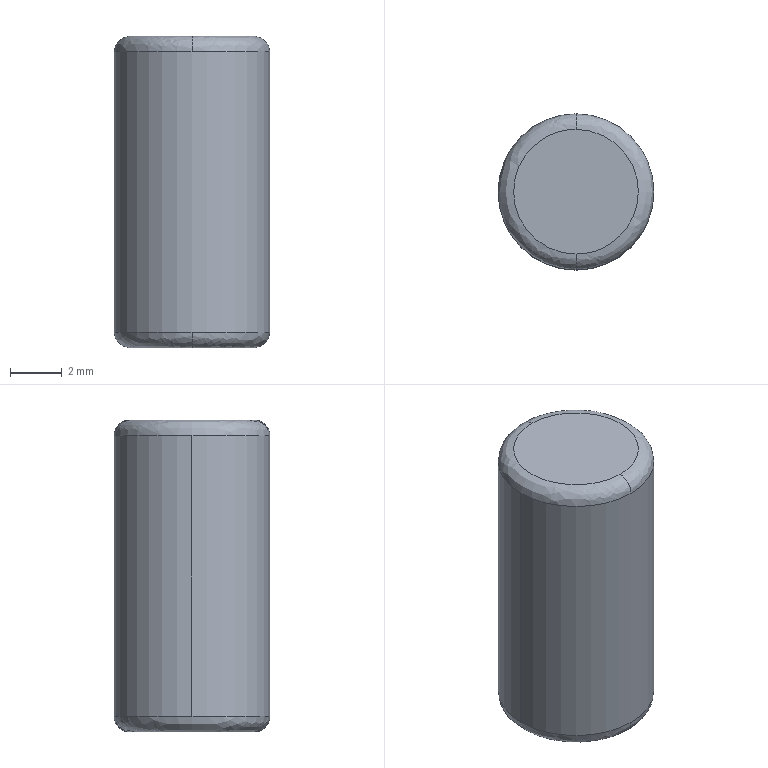Part | SolidWorks | features BaseBody 1 | 1 solid | 8 faces | box 6 x 6 x 12 mm | volume 336.497 mm3 | spline 4 | cylinder 2 | plane 2 | commonest cylinder face diameters 6 x2
STEP:
#1=CARTESIAN_POINT('',(442.747,1086.806,-452.745));
#2=VERTEX_POINT('',#1);
#3=CARTESIAN_POINT('',(445.747,1089.806,-452.745));
#4=VERTEX_POINT('',#3);
#5=CARTESIAN_POINT('',(442.747,1089.806,-452.745));
#6=DIRECTION('',(0.,0.,1.));
#7=DIRECTION('',(-1.,0.,0.));
#8=AXIS2_PLACEMENT_3D('',#5,#6,#7);
#9=CIRCLE('',#8,3.);
#10=EDGE_CURVE('',#2,#4,#9,.T.);
#11=ORIENTED_EDGE('',*,*,#10,.F.);
#12=CARTESIAN_POINT('',(442.747,1087.406,-453.345));
#13=VERTEX_POINT('',#12);
#14=CARTESIAN_POINT('',(442.747,1087.406,-452.745));
#15=DIRECTION('',(1.,0.,0.));
#16=DIRECTION('',(0.,-1.,0.));
#17=AXIS2_PLACEMENT_3D('',#14,#15,#16);
#18=CIRCLE('',#17,0.6);
#19=EDGE_CURVE('',#2,#13,#18,.T.);
#20=ORIENTED_EDGE('',*,*,#19,.T.);
#21=CARTESIAN_POINT('',(442.747,1092.206,-453.345));
#22=VERTEX_POINT('',#21);
#23=CARTESIAN_POINT('',(442.747,1087.406,-453.345));
#24=CARTESIAN_POINT('',(447.547,1087.406,-453.345));
#25=CARTESIAN_POINT('',(447.547,1092.206,-453.345));
#26=CARTESIAN_POINT('',(442.747,1092.206,-453.345));
#27=(BOUNDED_CURVE()B_SPLINE_CURVE(3,(#23,#24,#25,#26),.UNSPECIFIED.,.F.,.F.)B_SPLINE_CURVE_WITH_KNOTS((4,4),(0.,1.),.UNSPECIFIED.)CURVE()GEOMETRIC_REPRESENTATION_ITEM()RATIONAL_B_SPLINE_CURVE((1.,0.3333,0.3333,1.))REPRESENTATION_ITEM(''));
#28=EDGE_CURVE('',#13,#22,#27,.T.);
#29=ORIENTED_EDGE('',*,*,#28,.T.);
#30=CARTESIAN_POINT('',(442.747,1092.806,-452.745));
#31=VERTEX_POINT('',#30);
#32=CARTESIAN_POINT('',(442.747,1092.206,-452.745));
#33=DIRECTION('',(-1.,0.,0.));
#34=DIRECTION('',(0.,1.,0.));
#35=AXIS2_PLACEMENT_3D('',#32,#33,#34);
#36=CIRCLE('',#35,0.6);
#37=EDGE_CURVE('',#31,#22,#36,.T.);
#38=ORIENTED_EDGE('',*,*,#37,.F.);
#39=CARTESIAN_POINT('',(442.747,1089.806,-452.745));
#40=DIRECTION('',(0.,0.,1.));
#41=DIRECTION('',(-1.,0.,0.));
#42=AXIS2_PLACEMENT_3D('',#39,#40,#41);
#43=CIRCLE('',#42,3.);
#44=EDGE_CURVE('',#4,#31,#43,.T.);
#45=ORIENTED_EDGE('',*,*,#44,.F.);
#46=EDGE_LOOP('',(#11,#20,#29,#38,#45));
#47=FACE_OUTER_BOUND('',#46,.T.);
#48=CARTESIAN_POINT('',(442.747,1086.806,-452.745));
#49=CARTESIAN_POINT('',(448.747,1086.806,-452.745));
#50=CARTESIAN_POINT('',(448.747,1092.806,-452.745));
#51=CARTESIAN_POINT('',(442.747,1092.806,-452.745));
#52=CARTESIAN_POINT('',(442.747,1086.806,-453.096));
#53=CARTESIAN_POINT('',(448.747,1086.806,-453.096));
#54=CARTESIAN_POINT('',(448.747,1092.806,-453.096));
#55=CARTESIAN_POINT('',(442.747,1092.806,-453.096));
#56=CARTESIAN_POINT('',(442.747,1087.054,-453.345));
#57=CARTESIAN_POINT('',(448.249,1087.054,-453.345));
#58=CARTESIAN_POINT('',(448.249,1092.557,-453.345));
#59=CARTESIAN_POINT('',(442.747,1092.557,-453.345));
#60=CARTESIAN_POINT('',(442.747,1087.406,-453.345));
#61=CARTESIAN_POINT('',(447.547,1087.406,-453.345));
#62=CARTESIAN_POINT('',(447.547,1092.206,-453.345));
#63=CARTESIAN_POINT('',(442.747,1092.206,-453.345));
#64=(BOUNDED_SURFACE()B_SPLINE_SURFACE(3,3,((#48,#49,#50,#51),(#52,#53,#54,#55),(#56,#57,#58,#59),(#60,#61,#62,#63)),.UNSPECIFIED.,.F.,.F.,.F.)B_SPLINE_SURFACE_WITH_KNOTS((4,4),(4,4),(0.,1.),(0.,1.),.UNSPECIFIED.)GEOMETRIC_REPRESENTATION_ITEM()RATIONAL_B_SPLINE_SURFACE(((1.,0.3333,0.3333,1.),(0.8047,0.2682,0.2682,0.8047),(0.8047,0.2682,0.2682,0.8047),(1.,0.3333,0.3333,1.)))REPRESENTATION_ITEM('')SURFACE());
#65=ADVANCED_FACE('',(#47),#64,.T.);
#66=CARTESIAN_POINT('',(442.747,1092.206,-441.345));
#67=VERTEX_POINT('',#66);
#68=CARTESIAN_POINT('',(442.747,1087.406,-441.345));
#69=VERTEX_POINT('',#68);
#70=CARTESIAN_POINT('',(442.747,1092.206,-441.345));
#71=CARTESIAN_POINT('',(447.547,1092.206,-441.345));
#72=CARTESIAN_POINT('',(447.547,1087.406,-441.345));
#73=CARTESIAN_POINT('',(442.747,1087.406,-441.345));
#74=(BOUNDED_CURVE()B_SPLINE_CURVE(3,(#70,#71,#72,#73),.UNSPECIFIED.,.F.,.F.)B_SPLINE_CURVE_WITH_KNOTS((4,4),(0.,1.),.UNSPECIFIED.)CURVE()GEOMETRIC_REPRESENTATION_ITEM()RATIONAL_B_SPLINE_CURVE((1.,0.3333,0.3333,1.))REPRESENTATION_ITEM(''));
#75=EDGE_CURVE('',#67,#69,#74,.T.);
#76=ORIENTED_EDGE('',*,*,#75,.T.);
#77=CARTESIAN_POINT('',(442.747,1086.806,-441.945));
#78=VERTEX_POINT('',#77);
#79=CARTESIAN_POINT('',(442.747,1087.406,-441.945));
#80=DIRECTION('',(1.,0.,0.));
#81=DIRECTION('',(0.,-1.,0.));
#82=AXIS2_PLACEMENT_3D('',#79,#80,#81);
#83=CIRCLE('',#82,0.6);
#84=EDGE_CURVE('',#69,#78,#83,.T.);
#85=ORIENTED_EDGE('',*,*,#84,.T.);
#86=CARTESIAN_POINT('',(445.747,1089.806,-441.945));
#87=VERTEX_POINT('',#86);
#88=CARTESIAN_POINT('',(442.747,1089.806,-441.945));
#89=DIRECTION('',(0.,0.,-1.));
#90=DIRECTION('',(-1.,0.,0.));
#91=AXIS2_PLACEMENT_3D('',#88,#89,#90);
#92=CIRCLE('',#91,3.);
#93=EDGE_CURVE('',#87,#78,#92,.T.);
#94=ORIENTED_EDGE('',*,*,#93,.F.);
#95=CARTESIAN_POINT('',(442.747,1092.806,-441.945));
#96=VERTEX_POINT('',#95);
#97=CARTESIAN_POINT('',(442.747,1089.806,-441.945));
#98=DIRECTION('',(0.,0.,-1.));
#99=DIRECTION('',(-1.,0.,0.));
#100=AXIS2_PLACEMENT_3D('',#97,#98,#99);
#101=CIRCLE('',#100,3.);
#102=EDGE_CURVE('',#96,#87,#101,.T.);
#103=ORIENTED_EDGE('',*,*,#102,.F.);
#104=CARTESIAN_POINT('',(442.747,1092.206,-441.945));
#105=DIRECTION('',(-1.,0.,0.));
#106=DIRECTION('',(0.,1.,0.));
#107=AXIS2_PLACEMENT_3D('',#104,#105,#106);
#108=CIRCLE('',#107,0.6);
#109=EDGE_CURVE('',#67,#96,#108,.T.);
#110=ORIENTED_EDGE('',*,*,#109,.F.);
#111=EDGE_LOOP('',(#76,#85,#94,#103,#110));
#112=FACE_OUTER_BOUND('',#111,.T.);
#113=CARTESIAN_POINT('',(442.747,1087.406,-441.345));
#114=CARTESIAN_POINT('',(447.547,1087.406,-441.345));
#115=CARTESIAN_POINT('',(447.547,1092.206,-441.345));
#116=CARTESIAN_POINT('',(442.747,1092.206,-441.345));
#117=CARTESIAN_POINT('',(442.747,1087.054,-441.345));
#118=CARTESIAN_POINT('',(448.249,1087.054,-441.345));
#119=CARTESIAN_POINT('',(448.249,1092.557,-441.345));
#120=CARTESIAN_POINT('',(442.747,1092.557,-441.345));
#121=CARTESIAN_POINT('',(442.747,1086.806,-441.593));
#122=CARTESIAN_POINT('',(448.747,1086.806,-441.593));
#123=CARTESIAN_POINT('',(448.747,1092.806,-441.593));
#124=CARTESIAN_POINT('',(442.747,1092.806,-441.593));
#125=CARTESIAN_POINT('',(442.747,1086.806,-441.945));
#126=CARTESIAN_POINT('',(448.747,1086.806,-441.945));
#127=CARTESIAN_POINT('',(448.747,1092.806,-441.945));
#128=CARTESIAN_POINT('',(442.747,1092.806,-441.945));
#129=(BOUNDED_SURFACE()B_SPLINE_SURFACE(3,3,((#113,#114,#115,#116),(#117,#118,#119,#120),(#121,#122,#123,#124),(#125,#126,#127,#128)),.UNSPECIFIED.,.F.,.F.,.F.)B_SPLINE_SURFACE_WITH_KNOTS((4,4),(4,4),(0.,1.),(0.,1.),.UNSPECIFIED.)GEOMETRIC_REPRESENTATION_ITEM()RATIONAL_B_SPLINE_SURFACE(((1.,0.3333,0.3333,1.),(0.8047,0.2682,0.2682,0.8047),(0.8047,0.2682,0.2682,0.8047),(1.,0.3333,0.3333,1.)))REPRESENTATION_ITEM('')SURFACE());
#130=ADVANCED_FACE('',(#112),#129,.T.);
#131=CARTESIAN_POINT('',(439.747,1089.806,-441.945));
#132=VERTEX_POINT('',#131);
#133=CARTESIAN_POINT('',(442.747,1089.806,-441.945));
#134=DIRECTION('',(0.,0.,-1.));
#135=DIRECTION('',(-1.,0.,0.));
#136=AXIS2_PLACEMENT_3D('',#133,#134,#135);
#137=CIRCLE('',#136,3.);
#138=EDGE_CURVE('',#132,#96,#137,.T.);
#139=ORIENTED_EDGE('',*,*,#138,.T.);
#140=ORIENTED_EDGE('',*,*,#102,.T.);
#141=CARTESIAN_POINT('',(445.747,1089.806,-441.345));
#142=DIRECTION('',(0.,0.,-1.));
#143=VECTOR('',#142,1000.);
#144=LINE('',#141,#143);
#145=EDGE_CURVE('',#87,#4,#144,.T.);
#146=ORIENTED_EDGE('',*,*,#145,.T.);
#147=ORIENTED_EDGE('',*,*,#44,.T.);
#148=CARTESIAN_POINT('',(439.747,1089.806,-452.745));
#149=VERTEX_POINT('',#148);
#150=CARTESIAN_POINT('',(442.747,1089.806,-452.745));
#151=DIRECTION('',(0.,0.,1.));
#152=DIRECTION('',(-1.,0.,0.));
#153=AXIS2_PLACEMENT_3D('',#150,#151,#152);
#154=CIRCLE('',#153,3.);
#155=EDGE_CURVE('',#31,#149,#154,.T.);
#156=ORIENTED_EDGE('',*,*,#155,.T.);
#157=CARTESIAN_POINT('',(439.747,1089.806,-441.345));
#158=DIRECTION('',(0.,0.,-1.));
#159=VECTOR('',#158,1000.);
#160=LINE('',#157,#159);
#161=EDGE_CURVE('',#132,#149,#160,.T.);
#162=ORIENTED_EDGE('',*,*,#161,.F.);
#163=EDGE_LOOP('',(#139,#140,#146,#147,#156,#162));
#164=FACE_OUTER_BOUND('',#163,.T.);
#165=CARTESIAN_POINT('',(442.747,1089.806,-441.345));
#166=DIRECTION('',(0.,0.,-1.));
#167=DIRECTION('',(-1.,0.,0.));
#168=AXIS2_PLACEMENT_3D('',#165,#166,#167);
#169=CYLINDRICAL_SURFACE('',#168,3.);
#170=ADVANCED_FACE('',(#164),#169,.T.);
#171=ORIENTED_EDGE('',*,*,#145,.F.);
#172=ORIENTED_EDGE('',*,*,#93,.T.);
#173=CARTESIAN_POINT('',(442.747,1089.806,-441.945));
#174=DIRECTION('',(0.,0.,-1.));
#175=DIRECTION('',(-1.,0.,0.));
#176=AXIS2_PLACEMENT_3D('',#173,#174,#175);
#177=CIRCLE('',#176,3.);
#178=EDGE_CURVE('',#78,#132,#177,.T.);
#179=ORIENTED_EDGE('',*,*,#178,.T.);
#180=ORIENTED_EDGE('',*,*,#161,.T.);
#181=CARTESIAN_POINT('',(442.747,1089.806,-452.745));
#182=DIRECTION('',(0.,0.,1.));
#183=DIRECTION('',(-1.,0.,0.));
#184=AXIS2_PLACEMENT_3D('',#181,#182,#183);
#185=CIRCLE('',#184,3.);
#186=EDGE_CURVE('',#149,#2,#185,.T.);
#187=ORIENTED_EDGE('',*,*,#186,.T.);
#188=ORIENTED_EDGE('',*,*,#10,.T.);
#189=EDGE_LOOP('',(#171,#172,#179,#180,#187,#188));
#190=FACE_OUTER_BOUND('',#189,.T.);
#191=CARTESIAN_POINT('',(442.747,1089.806,-441.345));
#192=DIRECTION('',(0.,0.,-1.));
#193=DIRECTION('',(-1.,0.,0.));
#194=AXIS2_PLACEMENT_3D('',#191,#192,#193);
#195=CYLINDRICAL_SURFACE('',#194,3.);
#196=ADVANCED_FACE('',(#190),#195,.T.);
#197=ORIENTED_EDGE('',*,*,#19,.F.);
#198=ORIENTED_EDGE('',*,*,#186,.F.);
#199=ORIENTED_EDGE('',*,*,#155,.F.);
#200=ORIENTED_EDGE('',*,*,#37,.T.);
#201=CARTESIAN_POINT('',(442.747,1092.206,-453.345));
#202=CARTESIAN_POINT('',(437.947,1092.206,-453.345));
#203=CARTESIAN_POINT('',(437.947,1087.406,-453.345));
#204=CARTESIAN_POINT('',(442.747,1087.406,-453.345));
#205=(BOUNDED_CURVE()B_SPLINE_CURVE(3,(#201,#202,#203,#204),.UNSPECIFIED.,.F.,.F.)B_SPLINE_CURVE_WITH_KNOTS((4,4),(0.,1.),.UNSPECIFIED.)CURVE()GEOMETRIC_REPRESENTATION_ITEM()RATIONAL_B_SPLINE_CURVE((1.,0.3333,0.3333,1.))REPRESENTATION_ITEM(''));
#206=EDGE_CURVE('',#22,#13,#205,.T.);
#207=ORIENTED_EDGE('',*,*,#206,.T.);
#208=EDGE_LOOP('',(#197,#198,#199,#200,#207));
#209=FACE_OUTER_BOUND('',#208,.T.);
#210=CARTESIAN_POINT('',(442.747,1092.806,-452.745));
#211=CARTESIAN_POINT('',(436.747,1092.806,-452.745));
#212=CARTESIAN_POINT('',(436.747,1086.806,-452.745));
#213=CARTESIAN_POINT('',(442.747,1086.806,-452.745));
#214=CARTESIAN_POINT('',(442.747,1092.806,-453.096));
#215=CARTESIAN_POINT('',(436.747,1092.806,-453.096));
#216=CARTESIAN_POINT('',(436.747,1086.806,-453.096));
#217=CARTESIAN_POINT('',(442.747,1086.806,-453.096));
#218=CARTESIAN_POINT('',(442.747,1092.557,-453.345));
#219=CARTESIAN_POINT('',(437.244,1092.557,-453.345));
#220=CARTESIAN_POINT('',(437.244,1087.054,-453.345));
#221=CARTESIAN_POINT('',(442.747,1087.054,-453.345));
#222=CARTESIAN_POINT('',(442.747,1092.206,-453.345));
#223=CARTESIAN_POINT('',(437.947,1092.206,-453.345));
#224=CARTESIAN_POINT('',(437.947,1087.406,-453.345));
#225=CARTESIAN_POINT('',(442.747,1087.406,-453.345));
#226=(BOUNDED_SURFACE()B_SPLINE_SURFACE(3,3,((#210,#211,#212,#213),(#214,#215,#216,#217),(#218,#219,#220,#221),(#222,#223,#224,#225)),.UNSPECIFIED.,.F.,.F.,.T.)B_SPLINE_SURFACE_WITH_KNOTS((4,4),(4,4),(0.,1.),(0.,1.),.UNSPECIFIED.)GEOMETRIC_REPRESENTATION_ITEM()RATIONAL_B_SPLINE_SURFACE(((1.,0.3333,0.3333,1.),(0.8047,0.2682,0.2682,0.8047),(0.8047,0.2682,0.2682,0.8047),(1.,0.3333,0.3333,1.)))REPRESENTATION_ITEM('')SURFACE());
#227=ADVANCED_FACE('',(#209),#226,.T.);
#228=ORIENTED_EDGE('',*,*,#84,.F.);
#229=CARTESIAN_POINT('',(442.747,1087.406,-441.345));
#230=CARTESIAN_POINT('',(437.947,1087.406,-441.345));
#231=CARTESIAN_POINT('',(437.947,1092.206,-441.345));
#232=CARTESIAN_POINT('',(442.747,1092.206,-441.345));
#233=(BOUNDED_CURVE()B_SPLINE_CURVE(3,(#229,#230,#231,#232),.UNSPECIFIED.,.F.,.T.)B_SPLINE_CURVE_WITH_KNOTS((4,4),(0.,1.),.UNSPECIFIED.)CURVE()GEOMETRIC_REPRESENTATION_ITEM()RATIONAL_B_SPLINE_CURVE((1.,0.3333,0.3333,1.))REPRESENTATION_ITEM(''));
#234=EDGE_CURVE('',#69,#67,#233,.T.);
#235=ORIENTED_EDGE('',*,*,#234,.T.);
#236=ORIENTED_EDGE('',*,*,#109,.T.);
#237=ORIENTED_EDGE('',*,*,#138,.F.);
#238=ORIENTED_EDGE('',*,*,#178,.F.);
#239=EDGE_LOOP('',(#228,#235,#236,#237,#238));
#240=FACE_OUTER_BOUND('',#239,.T.);
#241=CARTESIAN_POINT('',(442.747,1092.206,-441.345));
#242=CARTESIAN_POINT('',(437.947,1092.206,-441.345));
#243=CARTESIAN_POINT('',(437.947,1087.406,-441.345));
#244=CARTESIAN_POINT('',(442.747,1087.406,-441.345));
#245=CARTESIAN_POINT('',(442.747,1092.557,-441.345));
#246=CARTESIAN_POINT('',(437.244,1092.557,-441.345));
#247=CARTESIAN_POINT('',(437.244,1087.054,-441.345));
#248=CARTESIAN_POINT('',(442.747,1087.054,-441.345));
#249=CARTESIAN_POINT('',(442.747,1092.806,-441.593));
#250=CARTESIAN_POINT('',(436.747,1092.806,-441.593));
#251=CARTESIAN_POINT('',(436.747,1086.806,-441.593));
#252=CARTESIAN_POINT('',(442.747,1086.806,-441.593));
#253=CARTESIAN_POINT('',(442.747,1092.806,-441.945));
#254=CARTESIAN_POINT('',(436.747,1092.806,-441.945));
#255=CARTESIAN_POINT('',(436.747,1086.806,-441.945));
#256=CARTESIAN_POINT('',(442.747,1086.806,-441.945));
#257=(BOUNDED_SURFACE()B_SPLINE_SURFACE(3,3,((#241,#242,#243,#244),(#245,#246,#247,#248),(#249,#250,#251,#252),(#253,#254,#255,#256)),.UNSPECIFIED.,.F.,.F.,.T.)B_SPLINE_SURFACE_WITH_KNOTS((4,4),(4,4),(0.,1.),(0.,1.),.UNSPECIFIED.)GEOMETRIC_REPRESENTATION_ITEM()RATIONAL_B_SPLINE_SURFACE(((1.,0.3333,0.3333,1.),(0.8047,0.2682,0.2682,0.8047),(0.8047,0.2682,0.2682,0.8047),(1.,0.3333,0.3333,1.)))REPRESENTATION_ITEM('')SURFACE());
#258=ADVANCED_FACE('',(#240),#257,.T.);
#259=ORIENTED_EDGE('',*,*,#28,.F.);
#260=ORIENTED_EDGE('',*,*,#206,.F.);
#261=EDGE_LOOP('',(#259,#260));
#262=FACE_OUTER_BOUND('',#261,.T.);
#263=CARTESIAN_POINT('',(442.747,1089.806,-453.345));
#264=DIRECTION('',(0.,0.,1.));
#265=DIRECTION('',(1.,0.,0.));
#266=AXIS2_PLACEMENT_3D('',#263,#264,#265);
#267=PLANE('',#266);
#268=ADVANCED_FACE('',(#262),#267,.F.);
#269=ORIENTED_EDGE('',*,*,#75,.F.);
#270=ORIENTED_EDGE('',*,*,#234,.F.);
#271=EDGE_LOOP('',(#269,#270));
#272=FACE_OUTER_BOUND('',#271,.T.);
#273=CARTESIAN_POINT('',(442.747,1089.806,-441.345));
#274=DIRECTION('',(0.,0.,1.));
#275=DIRECTION('',(1.,0.,0.));
#276=AXIS2_PLACEMENT_3D('',#273,#274,#275);
#277=PLANE('',#276);
#278=ADVANCED_FACE('',(#272),#277,.T.);
#279=CLOSED_SHELL('',(#65,#130,#170,#196,#227,#258,#268,#278));
#280=MANIFOLD_SOLID_BREP('',#279);
#281=CARTESIAN_POINT('',(0.,0.,0.));
#282=DIRECTION('',(0.,0.,1.));
#283=DIRECTION('',(1.,0.,0.));
#284=AXIS2_PLACEMENT_3D('',#281,#282,#283);
#285=(LENGTH_UNIT()NAMED_UNIT(*)SI_UNIT(.MILLI.,.METRE.));
#286=UNCERTAINTY_MEASURE_WITH_UNIT(LENGTH_MEASURE(0.00001),#285,'','');
#287=(NAMED_UNIT(*)PLANE_ANGLE_UNIT()SI_UNIT($,.RADIAN.));
#288=(NAMED_UNIT(*)SI_UNIT($,.STERADIAN.)SOLID_ANGLE_UNIT());
#289=(GEOMETRIC_REPRESENTATION_CONTEXT(3)GLOBAL_UNCERTAINTY_ASSIGNED_CONTEXT((#286))GLOBAL_UNIT_ASSIGNED_CONTEXT((#285,#287,#288))REPRESENTATION_CONTEXT('',''));
#290=ADVANCED_BREP_SHAPE_REPRESENTATION('',(#280,#284),#289);